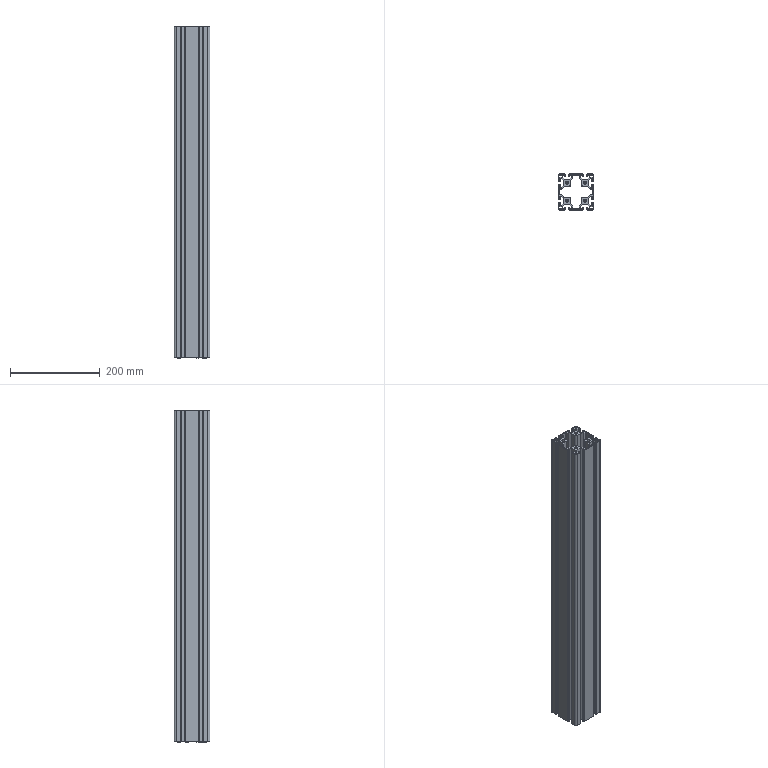Part | STEP file | LE-8-8080-S-OO_LE0313205357 | 1 solid | 380 faces | box 80 x 80 x 740 mm | volume 1300909 mm3 | plane 194 | cylinder 186 | commonest cylinder face diameters 0.6 x90 2 x52 0.4 x16 4 x8 6.8 x8 5 x4